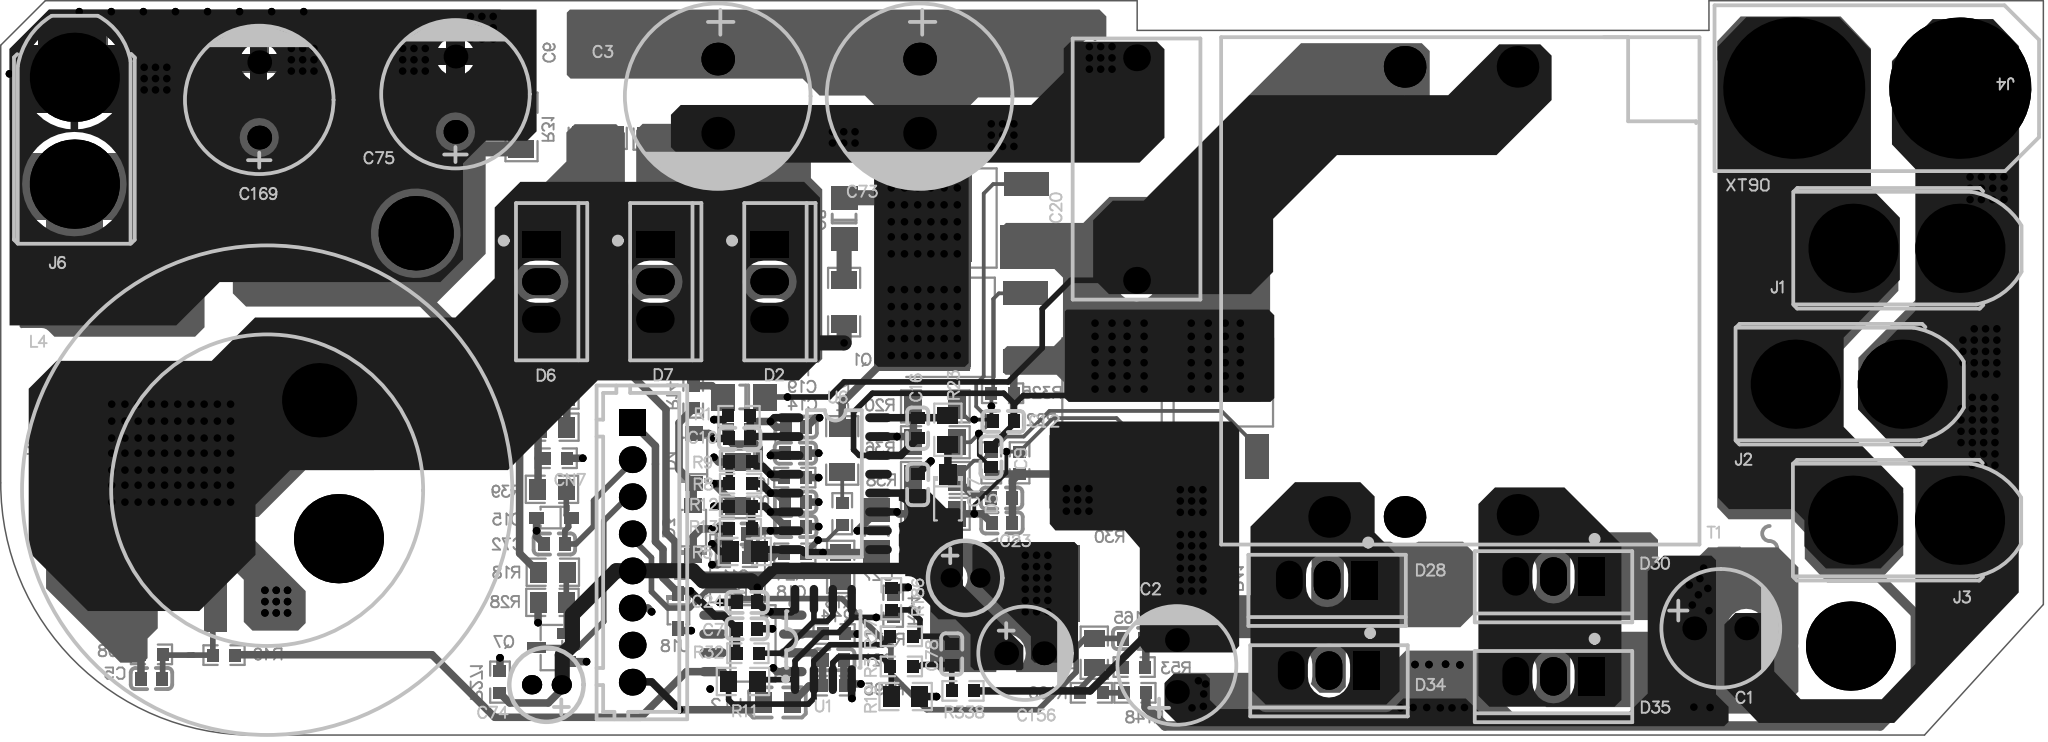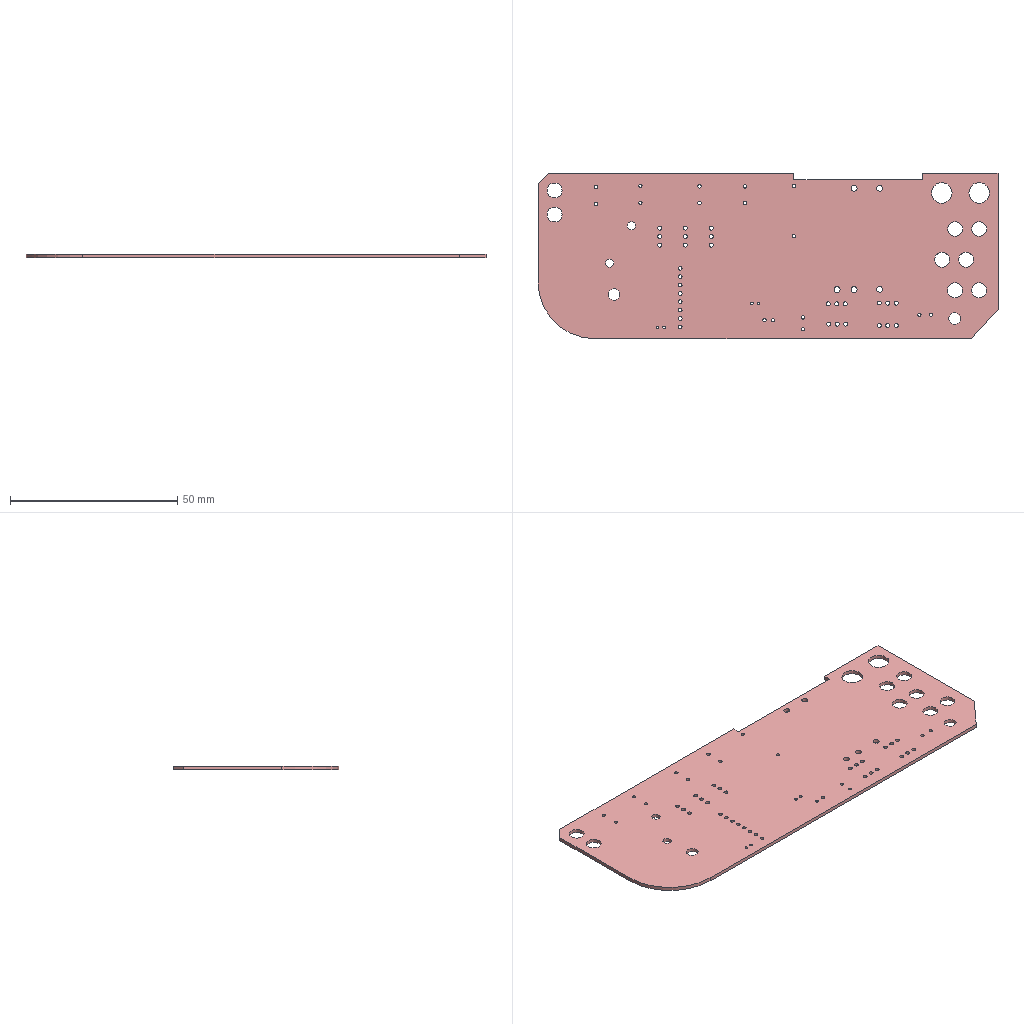Circuit board layout | Altium Designer | box 137.5 x 49.5 x 1.1 mm
Layer stack:
# Altium Designer layer stack of  (unit mm; dielectric type: 0 none, 1 core, 2 prepreg, 3 surface material)
index,name,kind,layer,copper_thickness_mm,dielectric_type,dielectric_thickness_mm,dielectric_material,dielectric_constant
0,Top Paste,other,,,,,,
1,Top Overlay,other,,,,,,
2,Top Solder,dielectric,,,3,0.0102,Solder Resist,3.5
3,Top Layer,copper,Top Layer,0.0356,,,,
4,Dielectric1,dielectric,,,1,0.32,FR-4,4.8
5,GND02,copper,GND02,0.0356,,,,
6,Dielectric2,dielectric,,,2,0.32,FR-4,4.8
7,PWR03,copper,PWR03,0.0356,,,,
8,Dielectric3,dielectric,,,1,0.32,FR-4,4.8
9,Bottom Layer,copper,Bottom Layer,0.0356,,,,
10,Bottom Solder,dielectric,,,3,0.0102,Solder Resist,3.5
11,Bottom Overlay,other,,,,,,
12,Bottom Paste,other,,,,,,
# drill layer pairs: low layer,high layer
drill_pair,Top Layer,Bottom Layer
Part placement:
Designator,Comment,Layer,Footprint,Center-X(mm),Center-Y(mm),Rotation
D7,SBD20C200T,TopLayer,TO-220-3_L10.0-W4.5-P2.54-L,44.576,29.997,270
D6,SBD20C200T,TopLayer,TO-220-3_L10.0-W4.5-P2.54-L,36.893,29.997,270
D2,SBD20C200T,TopLayer,TO-220-3_L10.0-W4.5-P2.54-L,52.26,29.997,270
C24,100nF,TopLayer,C0603,50.735,8.382,180
U1,EG358,TopLayer,SOIC-8_L5.0-W4.0-P1.27-LS6.0-BL,55.88,5.88,360
R32,1K,TopLayer,R0603,50.8,4.953,180
R11,100K,TopLayer,R0805,50.469,3.048,180
D1,MM3Z3V3_C123917,BottomLayer,SOD-323_L1.8-W1.3-LS2.5-RD,46.126,7.802,270
C23,22uF,TopLayer,CAP-TH_BD5.0-P2.00-D0.8-FD,65.421,10.033,360
J3,XT60,TopLayer,CONN-TH_XT60UPB-F,128.765,13.919,180
J4,XT60HOLE,TopLayer,XT90N,126.792,43.041,180
R13,,TopLayer,R0603,50.292,13.335,360
R12,,TopLayer,R0603,50.301,14.859,360
R9,3.65K,TopLayer,R0603,50.301,17.907,180
R8,,TopLayer,R0603,50.309,16.383,360
R1,1.5M,TopLayer,R0603,50.204,20.955,360
C10,220nF,TopLayer,C0603,50.257,19.431,360
L4,330uH,TopLayer,200W-TMS330060A,25.189,27.635,60
J2,XT60,TopLayer,CONN-TH_XT60UPB-F,124.904,23.089,180
J1,XT60,TopLayer,CONN-TH_XT60UPB-F,128.789,32.249,180
CN7,HX25003-8A,TopLayer,CONN-TH_8P-P2.50_HX25003-8A,43.015,11.751,90
C2,390uF,TopLayer,CAP-TH_BD8.0-P3.50-D0.6-FD,79.68,4.092,90
C3,560uF,TopLayer,CAP-TH_BD12.5-P5.00-D0.6-FD,48.768,42.505,270
C20,680nF,TopLayer,CAP-TH_L17.5-W8.5-P15.00-D0.8,76.962,37.592,90
C75,390uF,TopLayer,CAP-TH_BD10.0-P5.00-D1.0-FD,31.115,42.635,90
C169,390uF,TopLayer,CAP-TH_BD10.0-P5.00-D1.0-FD,17.907,42.254,90
R3,,TopLayer,R0603,61.13,4.064,360
R27,,TopLayer,R0603,61.13,6.096,360
R19,100K,TopLayer,R0805,61.418,2.032,360
U6,EG6599,TopLayer,SO-16_L10.0-W4.0-P1.27-LS6.2-BL,56.621,16.383,270
C73,560uF,TopLayer,CAP-TH_BD12.5-P5.00-D0.6-FD,62.357,42.505,270
D28,SBT40100VCT,TopLayer,TO-220-3_L10.0-W4.5-P2.54-L,89.789,9.886,180
D30,SBT40100VCT,TopLayer,TO-220-3_L10.0-W4.5-P2.54-L,105.029,10.13,180
D34,SBT40100VCT,TopLayer,TO-220-3_L10.0-W4.5-P2.54-L,89.916,3.79,180
D35,SBT40100VCT,TopLayer,TO-220-3_L10.0-W4.5-P2.54-L,105.029,3.399,180
J6,6A,TopLayer,CONN-TH_XT60UPB-F,5.461,40.176,270
C1,390uF,TopLayer,CAP-TH_BD8.0-P3.50-D0.6-FD,116.253,6.629,360
T1,,TopLayer,PQ3230_3:2:2-N,96.266,29.312,180
R338,1,TopLayer,R0603,65.278,2.413,360
R186,1,TopLayer,R0603,60.452,8.627,90
R5,,TopLayer,R0805,50.589,11.811,360
C78,100nF,TopLayer,C0603,64.516,4.891,270
C7,1nF,TopLayer,C0603,50.735,6.604,180
R23,,TopLayer,R0805,64.262,20.016,270
C17,100nF,TopLayer,C0603,62.23,16.321,270
C16,100nF,TopLayer,C0603,62.23,20.128,90
D5,FR107_C2760867,TopLayer,SOD-123FL_L2.7-W1.8-LS3.8-RD,64.262,15.283,270
C156,220uF,TopLayer,CAP-TH_BD6.3-P2.50-D1.0-FD,69.459,4.953,360
R47,,BottomLayer,R1206,57.277,28.62,90
R46,,BottomLayer,R2512,52.578,42.806,90
R43,,BottomLayer,R2512,115.004,2.972,360
R41,,BottomLayer,R2512,83.871,4.757,270
R34,1K,BottomLayer,R0603,60.579,8.119,90
R33,,BottomLayer,R2512,113.632,10.109,360
R10,,BottomLayer,R2512,97.384,5.824,270
Q3,CRSS042N10N,BottomLayer,TO-263-3_L10.2-W10.7-P5.08-LS16.2-TL,12.421,13.26,90
Q1,NCEP1520K,BottomLayer,TO-252-2_L6.6-W6.1-P4.57-LS9.9-BR-CW,66.04,26.924,360
R20,10,BottomLayer,R1206,63.418,21.59,360
R325,30K,BottomLayer,R0603,67.945,22.479,360
C15,NC,BottomLayer,C1206,50.546,22.225,180
R21,10,BottomLayer,R1206,63.418,14.351,360
R22,30K,BottomLayer,R0603,67.936,20.574,360
Q5,NCEP1520K,BottomLayer,TO-252-2_L6.6-W6.1-P4.57-LS9.9-BR-CW,66.162,34.29,360
R14,,BottomLayer,R0603,47.117,22.216,270
R25,,BottomLayer,R2512,40.691,42.882,90
R42,,BottomLayer,R2512,45.06,42.831,90
R98,30K,BottomLayer,R0603,10.651,4.877,360
R49,10,BottomLayer,R0603,15.536,4.826,360
R7,,BottomLayer,R0603,53.955,16.793,360
R6,3K,BottomLayer,R0603,50.204,20.066,360
R4,,BottomLayer,R0603,50.029,11.43,360
Q7,MMBT3904,BottomLayer,SOT-23-3_L2.9-W1.3-P1.90-LS2.4-BR,37.576,5.334,360
C72,100nF,BottomLayer,C0603,37.781,12.319,360
C19,1nF,BottomLayer,C0603,54.009,18.444,360
C18,470pF,BottomLayer,C0603,54.009,13.491,180
C14,1nF,BottomLayer,C0603,54.009,15.142,180
C13,2.2uF,BottomLayer,C0603,54.037,20.193,180
C11,1uF,BottomLayer,C0603,50.072,12.982,180
C8,2.2nF,BottomLayer,C1206,57.277,34.257,90
C6,2.2nF,BottomLayer,C1206,35.56,45.596,90
C4,2.2nF,BottomLayer,C1206,4.648,13.668,270
D3,1N4148W_C388533,BottomLayer,SOD-123_L2.8-W1.8-LS3.7-RD,47.117,13.208,90
D4,1N4148W_C388533,BottomLayer,SOD-123_L2.8-W1.8-LS3.7-RD,47.193,18.076,90
F6,10A/200V,BottomLayer,FUSE-SMD_L6.1-W2.5,15.45,34.544,360
R2,,BottomLayer,R1206,4.648,19.081,270
R15,10K,BottomLayer,R1206,50.136,16.366,90
R16,,BottomLayer,R0603,57.15,14.36,270
R17,,BottomLayer,R1206,57.15,18.624,270
R24,,BottomLayer,R0603,53.959,11.684,180
R26,100K,BottomLayer,R0805,37.642,22.352,180
R28,,BottomLayer,R0805,37.642,8.382,360
R29,,BottomLayer,R0603,37.898,18.098,180
R31,,BottomLayer,R1206,35.56,40.431,90
R35,0,BottomLayer,R0805,37.642,20.193,360
R36,10,BottomLayer,R1206,63.418,19.177,360
R37,30K,BottomLayer,R0603,67.183,17.789,270
R39,,BottomLayer,R0805,37.61,16.002,180
D15,MM3Z3V3_C123917,BottomLayer,SOD-323_L1.8-W1.3-LS2.5-RD,37.749,14.097,180
R148,,BottomLayer,R0603,76.852,2.286,360
R106,30K,BottomLayer,R0603,73.923,2.286,360
R53,30K,BottomLayer,R0603,76.802,4.021,180
C165,100nF,BottomLayer,C0603,76.759,5.944,180
R40,,BottomLayer,R0805,74.117,4.987,90
Q6,NCEP1520K,BottomLayer,TO-252-2_L6.6-W6.1-P4.57-LS9.9-BR-CW,82.804,21.62,270
Q2,NCEP1520K,BottomLayer,TO-252-2_L6.6-W6.1-P4.57-LS9.9-BR-CW,75.311,21.615,270
R30,,BottomLayer,R2512,75.547,9.906,360
R38,10,BottomLayer,R1206,63.418,16.764,360
R18,100K,BottomLayer,R0805,37.669,10.414,180
R302,30K,BottomLayer,R0603,69.088,17.789,270
C21,220pF,BottomLayer,C0603,56.568,4.512,180
C74,22uF,TopLayer,CAP-TH_BD5.0-P2.00-D0.8-FD,37.238,2.829,180
R237,,BottomLayer,R0603,56.6,6.25,180
R271,,BottomLayer,R0603,34.112,3.006,270
R295,NC,BottomLayer,R0603,56.557,2.767,360
U18,EG3113,BottomLayer,SOP-8_L4.9-W3.9-P1.27-LS6.0-BL,51.139,5.615,270
C5,2.2nF,BottomLayer,C0603,10.645,3.242,180
C9,2.2nF,TopLayer,C0603,67.167,18.184,90
C12,2.2nF,TopLayer,C0603,68.012,20.576,360
C22,2.2nF,BottomLayer,C0603,67.885,15.416,360
C25,2.2nF,BottomLayer,C0603,67.91,13.739,360
F1,20A/200V,BottomLayer,FUSE-SMD_L6.1-W2.5,119.585,12.513,90
L12,BLM21PG300SN1D,BottomLayer,L0805,52.83,1.635,360
C27,10nF,BottomLayer,C1206,59.459,13.192,270
R44,,BottomLayer,R0805,57.046,10.77,270
Pad and via stacks:
# Altium Designer via and pad stacks of  (unit mm). Each distinct definition once, with the count of objects using it.
# via: kind,start_layer,end_layer,hole_mm,diameter_mm,mode(0 simple;1 top-mid-bottom;2 full stack),diameter_per_layer,count,example_net
# pad: kind,layer,hole_mm,hole_type(0 round;1 square;2 slot),plating,top_size,top_shape(1 round;2 rect;3 octagon;9 rounded rect),mid_size,bottom_size,mode,footprint,size_per_layer,count,example
pad,Top Layer,0,0,plated,0.8065x0.864,2,0.8065x0.864,0.8065x0.864,0,R0603,,20,R186.1
pad,Top Layer,0,0,plated,0.8x0.9,2,0.8x0.9,0.8x0.9,0,C0603,,16,C78.1
pad,Top Layer,0,0,plated,1.133x1.377,2,1.133x1.377,1.133x1.377,0,R0805,,8,R11.2
pad,Top Layer,0,0,plated,1.4x1.2,2,1.4x1.2,1.4x1.2,0,SOD-123FL_L2.7-W1.8-LS3.8-RD,,2,D5.1
pad,Top Layer,0,0,plated,0.6x1.8,1,0.6x1.8,0.6x1.8,0,SO-16_L10.0-W4.0-P1.27-LS6.2-BL,,16,U6.1
pad,Top Layer,0,0,plated,0.5684x1.95,1,0.5684x1.95,0.5684x1.95,0,SOIC-8_L5.0-W4.0-P1.27-LS6.0-BL,,8,U1.5
pad,Bottom Layer,0,0,plated,0.8065x0.864,2,0.8065x0.864,0.8065x0.864,0,R0603,,40,R271.2
pad,Bottom Layer,0,0,plated,1.8x1.6,2,1.8x1.6,1.8x1.6,0,C1206,,10,C27.1
pad,Bottom Layer,0,0,plated,1.133x1.377,2,1.133x1.377,1.133x1.377,0,R0805,,14,R44.1
pad,Bottom Layer,0,0,plated,1x0.75,2,1x0.75,1x0.75,0,SOD-323_L1.8-W1.3-LS2.5-RD,,4,D1.1
pad,Bottom Layer,0,0,plated,2.5x3,2,2.5x3,2.5x3,0,FUSE-SMD_L6.1-W2.5,,4,F1.2
pad,Bottom Layer,0,0,plated,0.8x0.9,2,0.8x0.9,0.8x0.9,0,C0603,,22,C22.1
pad,Bottom Layer,0,0,plated,1.133x1.377,2,1.133x1.377,1.133x1.377,0,L0805,,2,L12.1
pad,Bottom Layer,0,0,plated,1.282x3.456,2,1.282x3.456,1.282x3.456,0,R2512,,16,R43.2
pad,Bottom Layer,0,0,plated,1.208x1.701,2,1.208x1.701,1.208x1.701,0,R1206,,18,R47.2
pad,Bottom Layer,0,0,plated,0.95x1.15,2,0.95x1.15,0.95x1.15,0,SOD-123_L2.8-W1.8-LS3.7-RD,,4,D3.1
pad,Bottom Layer,0,0,plated,3x1.6,2,3x1.6,3x1.6,0,TO-252-2_L6.6-W6.1-P4.57-LS9.9-BR-CW,,8,Q5.1
pad,Bottom Layer,0,0,plated,6.2x5.8,2,6.2x5.8,6.2x5.8,0,TO-252-2_L6.6-W6.1-P4.57-LS9.9-BR-CW,,4,Q5.2
pad,Bottom Layer,0,0,plated,0.63x1.865,1,0.63x1.865,0.63x1.865,0,SOP-8_L4.9-W3.9-P1.27-LS6.0-BL,,8,U18.5
pad,Bottom Layer,0,0,plated,1.25x0.7,2,1.25x0.7,1.25x0.7,0,SOT-23-3_L2.9-W1.3-P1.90-LS2.4-BR,,3,Q7.1
pad,Bottom Layer,0,0,plated,10.7x8.38,2,10.7x8.38,10.7x8.38,0,TO-263-3_L10.2-W10.7-P5.08-LS16.2-TL,,1,Q3.2
pad,Bottom Layer,0,0,plated,1.5x3.504,2,1.5x3.504,1.5x3.504,0,TO-263-3_L10.2-W10.7-P5.08-LS16.2-TL,,2,Q3.3
pad,Multi-Layer,1.2,0,plated,1.8x2.6,2,1.8x2.6,1.8x2.6,0,TO-220-3_L10.0-W4.5-P2.54-L,,7,D2.1
pad,Multi-Layer,1.2,0,plated,1.8x2.6,1,1.8x2.6,1.8x2.6,0,TO-220-3_L10.0-W4.5-P2.54-L,,14,D2.3
pad,Multi-Layer,1,0,plated,1.6x1.6,1,1.6x1.6,1.6x1.6,0,CAP-TH_BD10.0-P5.00-D1.0-FD,,4,C75.2
pad,Multi-Layer,1.1,0,plated,2.2x2.2,1,2.2x2.2,2.2x2.2,0,CAP-TH_BD12.5-P5.00-D0.6-FD,,4,C3.2
pad,Multi-Layer,1,0,plated,1.6x1.6,1,1.6x1.6,1.6x1.6,0,CAP-TH_BD8.0-P3.50-D0.6-FD,,4,C2.1
pad,Multi-Layer,4.5,0,plated,6x6,1,6x6,6x6,0,CONN-TH_XT60UPB-F,,8,J1.1
pad,Multi-Layer,0.8,0,plated,1.3x1.3,1,1.3x1.3,1.3x1.3,0,CAP-TH_BD5.0-P2.00-D0.8-FD,,4,C23.2
pad,Multi-Layer,3.5,0,plated,6x6,1,6x6,6x6,0,,,2,0
pad,Multi-Layer,1,0,plated,1.6x1.6,1,1.6x1.6,1.6x1.6,0,CAP-TH_BD6.3-P2.50-D1.0-FD,,2,C156.2
pad,Multi-Layer,1,0,plated,1.8x1.8,1,1.8x1.8,1.8x1.8,0,CAP-TH_L17.5-W8.5-P15.00-D0.8,,2,C20.2
pad,Multi-Layer,1.1,0,plated,1.8x1.8,2,1.8x1.8,1.8x1.8,0,CONN-TH_8P-P2.50_HX25003-8A,,1,CN7.1
pad,Multi-Layer,1.1,0,plated,1.8x1.8,1,1.8x1.8,1.8x1.8,0,CONN-TH_8P-P2.50_HX25003-8A,,7,CN7.2
pad,Multi-Layer,2.5,0,plated,5x5,1,5x5,5x5,0,200W-TMS330060A,,2,L4.1
pad,Multi-Layer,1.8,0,plated,2.8x2.8,1,2.8x2.8,2.8x2.8,0,PQ3230 3:2:2-N,,5,T1.8
pad,Multi-Layer,6.2,0,plated,9.5x9.5,1,9.5x9.5,9.5x9.5,0,XT90N,,2,J4.1
via,Top Layer,Bottom Layer,0.254,0.508,0,,418,GND
via,Top Layer,Bottom Layer,0.3048,0.508,0,,24,NetC1_1
Copper pours:
name,layer,net,type(0 solid;1 hatched;2 none)
BottomLayer-No Net,Top Layer,LLC_I,0
BottomLayer-No Net,Top Layer,NetD30_1,0
BottomLayer-No Net,Top Layer,NetD28_1,0
BottomLayer-No Net,Top Layer,NetC1_1,0
BottomLayer-No Net,Top Layer,B+,0
BottomLayer-No Net,Top Layer,NetD2_1,0
BOTTOM-No Net,Top Layer,NetC3_1,0
BOTTOM-No Net,Top Layer,T1H,0
BOTTOM-No Net,Top Layer,GND,0
BOTTOM-No Net,Top Layer,+12V,0
BOTTOM-No Net,Top Layer,BAT-,0
BOTTOM-No Net,Top Layer,GND,0
BottomLayer-No Net,Top Layer,BAT-,0
BottomLayer-No Net,Top Layer,BAT-,0
BottomLayer-No Net,GND02,BAT-,0
BOTTOM-No Net,GND02,BAT-,0
BOTTOM-No Net,GND02,GND,0
BottomLayer-No Net,PWR03,B+,0
BottomLayer-No Net,PWR03,NetC1_1,0
BottomLayer-No Net,PWR03,BAT-,0
BottomLayer-No Net,PWR03,BAT-,0
BOTTOM-No Net,PWR03,NetC3_1,0
BOTTOM-No Net,PWR03,T1H,0
BOTTOM-No Net,PWR03,BAT-,0
BOTTOM-No Net,PWR03,GND,0
BOTTOM-No Net,PWR03,GND,0
BottomLayer-No Net,Bottom Layer,T1H,0
BottomLayer-No Net,Bottom Layer,NetC1_1,0
BottomLayer-No Net,Bottom Layer,B+,0
BottomLayer-No Net,Bottom Layer,NetD30_2,0
BottomLayer-No Net,Bottom Layer,NetD6_2,0
BottomLayer-No Net,Bottom Layer,NetD7_2,0
BottomLayer-No Net,Bottom Layer,NetD2_1,0
BottomLayer-No Net,Bottom Layer,BAT-,0
BottomLayer-No Net,Bottom Layer,NetD34_2,0
BottomLayer-No Net,Bottom Layer,BAT-,0
BottomLayer-No Net,Bottom Layer,BAT-,0
BottomLayer-No Net,Bottom Layer,NetD35_2,0
BottomLayer-No Net,Bottom Layer,NetD28_2,0
BOTTOM-No Net,Bottom Layer,,0
BOTTOM-No Net,Bottom Layer,PV+,0
BOTTOM-No Net,Bottom Layer,PV-OVP,0
BOTTOM-No Net,Bottom Layer,GND,0
BOTTOM-No Net,Bottom Layer,NetC3_1,0
BOTTOM-No Net,Bottom Layer,NetD2_2,0
BOTTOM-No Net,Bottom Layer,GND,0
Design rules, without the lines most boards share:
# Altium Designer design rules of  (exported by Altium Designer, unit mm)
# columns: name | kind | enabled | priority | scope1 | scope2 | descriptor | typed fields (field=value)
NetAntennae | 56 | enabled | 1 | All | All | Net Antennae (Tolerance=1mil) (All) |
SilkToSilkClearance | 55 | disabled | 1 | All | All | Silk to Silk (Clearance=10mil) (Disabled)(All),(All) |
SilkscreenOverComponentPads | 54 | disabled | 1 | IsPad | All | Silk To Solder Mask (Clearance=10mil) (Disabled)(IsPad),(All) |
MinimumSolderMaskSliver | 53 | disabled | 1 | All | All | Minimum Solder Mask Sliver (Gap=10mil) (Disabled)(All),(All) |
HoleToHoleClearance | 52 | disabled | 1 | All | All | Hole To Hole Clearance (Gap=10mil) (Disabled)(All),(All) | gap=0.254
DiffPairsRouting | 51 | enabled | 1 | All | All | Differential Pairs Uncoupled Length using the Gap Constraints (Min=10mil) (Max=10mil) (Prefered=10mil)  and Width Constraints (Min=15mil) (Max=15mil) (Prefered=15mil) (All) |
Height | 50 | disabled | 1 | All | All | Height Constraint (Min=0mil) (Max=1000mil) (Prefered=500mil) (Disabled)(All) | min_height=0 max_height=25.4
LayerPairs | 48 | disabled | 1 | All | All | Pads and Vias to follow the Drill pairs settings |
TestPointUsage | 44 | enabled | 1 | All | All | Fabrication Testpoint Usage (Valid =One Required, Allow multiple per net=No) (All) |
Testpoint | 43 | enabled | 1 | (IsPad And (OnTopLayer Or OnBottomLayer)) | All | Fabrication Testpoint Style (Under Component=Yes) ((IsPad And (OnTopLayer Or OnBottomLayer))) |
HoleSize | 42 | disabled | 1 | All | All | Hole Size Constraint (Min=1mil) (Max=100mil) (Disabled)(All) |
ComponentClearance | 24 | disabled | 1 | All | All | Component Clearance Constraint ( Horizontal Gap = 10mil, Vertical Gap = 10mil ) (Disabled)(All),(All)  | gap=0.254
PolygonConnect | 20 | enabled | 2 | All | All | Polygon Connect Rule(Direct Connect )(Conductor Width=35mil) (Relief Angle=90 Angle) (Entries=4) (Air Gap Width=10mil) (All),(All) | connect_style(0=relief,1=direct,2=none)=1 relief_conductor_width=0.889 relief_entries=4
PolygonConnect_1 | 20 | enabled | 1 | ISVIA | All | Polygon Connect Rule(Direct Connect )(Conductor Width=10mil) (Relief Angle=90 Angle) (Entries=4) (Air Gap Width=10mil) (ISVIA),(All) | connect_style(0=relief,1=direct,2=none)=1 relief_conductor_width=0.254 relief_entries=4
SolderMaskExpansion | 13 | enabled | 1 | All | All | Solder Mask Expansion (Expansion =2.5mil) (All) | expansion=0.0635
PlaneClearance | 12 | enabled | 1 | All | All | Power Plane Clearance (Clearance =12mil) (All) | clearance=0.3048
RoutingVias | 11 | enabled | 1 | All | All | Routing Via (MinHoleWidth=10mil) (MaxHoleWidth=12mil) (PreferredHoleWidth=10mil) (MinWidth=20mil) (MaxWidth=20mil) (PreferedWidth=20mil) (All) | via_min_hole=0.254 via_max_hole=0.3048 via_preferred_diameter=0.508 via_preferred_hole=0.254
PlaneConnect | 6 | enabled | 1 | All | All | Power Plane Connect Rule(Relief Connect )(Expansion=8mil) (Conductor Width=10mil) (Air Gap=10mil) (Entries=4) (All) | relief_conductor_width=0.254 relief_entries=4 relief_expansion=0.2032
Width | 2 | enabled | 1 | All | All | Width Constraint (Min=10mil) (Max=500mil) (Preferred=10mil) (All) |
all | 0 | enabled | 4 | All | All | Clearance Constraint (Gap=8mil) (All),(All) | gap=0.2032
40 | 0 | disabled | 1 | InNetClass('40') | All | Clearance Constraint (Gap=30mil) (Disabled)(InNetClass('40')),(All) | gap=0.762
Clearance_via | 0 | enabled | 2 | isvia | inpoly | Clearance Constraint (Gap=10mil) (isvia),(inpoly) | gap=0.254
Clearance | 0 | enabled | 3 | InPolygon | All | Clearance Constraint (Gap=20mil) (InPolygon),(All) | gap=0.508
Classes set for this board:
# Altium Designer classes of  (member kind: 0 net, 1 component, 2 from-to, 3 pad, 4 layer, 5 differential pair, 6 design channel, 7 polygon, 8 structure, 9 xSignal)
# columns: class name | member kind | superclass | members
200w_2022-10-14 | 1 | no | C1; C2; C3; C4; C6; C8; C10; C11; C13; C14; C15; C16; C17; C18; C19; C20; C23; C72; C73; C75; C78; C165; C169; CN7; D1; D3; D4; D5; D15; D28; D30; D34; D35; F6; J1; J2; J3; J4; J6; L4; Q1; Q2; Q3; Q5; Q6; Q7; R1; R2; R3; R4; R5; R6; R7; R8; R9; R11; R12; R13; R14; R15; R16; R17; R19; R20; R21; R22; R23; R24; R25; R26; R27; R28; R29; R30; R31; R19; R35; R36; R37; R38; R39; R40; R42; R49; R53; R98; R106; R148; R186; R302; R325; R338; T1; U1; U6; R32; Q1; Q2; Q3; Q5; Q6; C24; C7; D2; D6; D7; R10; R18; R33; R34; R41; R43; R46; R47; R302; C21; C74; C156; R237; R271; R295; U18; C5; C9; C12; C22; C25; F1; L12; C27; R44;